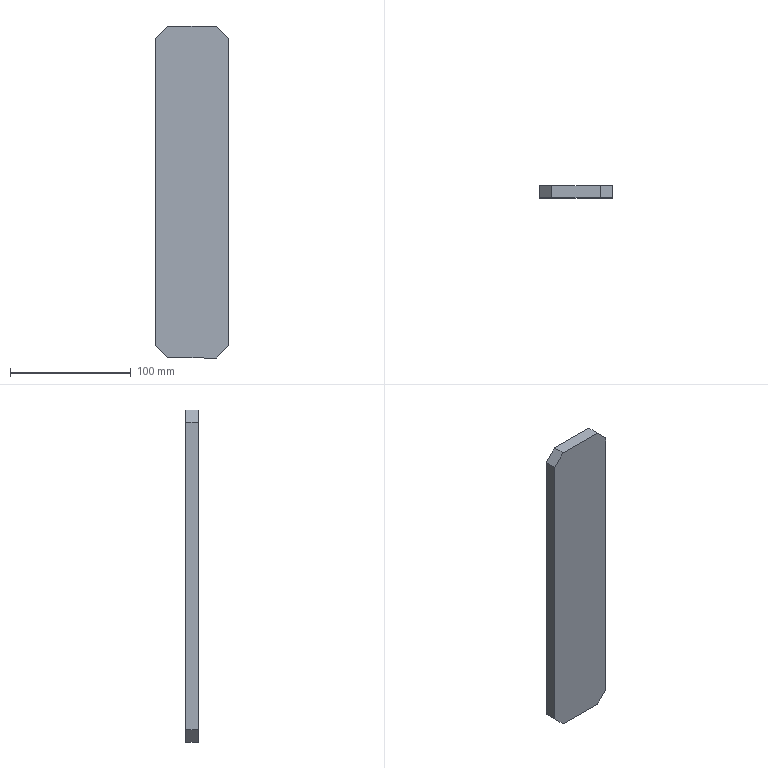Part | SolidWorks | features BaseBody 1 | 1 solid | 10 faces | box 60 x 10 x 275 mm | volume 163000 mm3 | plane 10
STEP:
#1=CARTESIAN_POINT('',(650.,52.,448.));
#2=VERTEX_POINT('',#1);
#3=CARTESIAN_POINT('',(640.,52.,438.));
#4=VERTEX_POINT('',#3);
#5=CARTESIAN_POINT('',(650.,52.,448.));
#6=DIRECTION('',(-0.7071,0.,-0.7071));
#7=VECTOR('',#6,1000.);
#8=LINE('',#5,#7);
#9=EDGE_CURVE('',#2,#4,#8,.T.);
#10=ORIENTED_EDGE('',*,*,#9,.T.);
#11=CARTESIAN_POINT('',(640.,52.,183.));
#12=VERTEX_POINT('',#11);
#13=CARTESIAN_POINT('',(640.,52.,-1110.));
#14=DIRECTION('',(0.,0.,-1.));
#15=VECTOR('',#14,1000.);
#16=LINE('',#13,#15);
#17=EDGE_CURVE('',#4,#12,#16,.T.);
#18=ORIENTED_EDGE('',*,*,#17,.T.);
#19=CARTESIAN_POINT('',(650.,52.,173.));
#20=VERTEX_POINT('',#19);
#21=CARTESIAN_POINT('',(640.,52.,183.));
#22=DIRECTION('',(0.7071,0.,-0.7071));
#23=VECTOR('',#22,1000.);
#24=LINE('',#21,#23);
#25=EDGE_CURVE('',#12,#20,#24,.T.);
#26=ORIENTED_EDGE('',*,*,#25,.T.);
#27=CARTESIAN_POINT('',(690.,52.,173.));
#28=VERTEX_POINT('',#27);
#29=CARTESIAN_POINT('',(1039.958,52.,173.));
#30=DIRECTION('',(1.,0.,0.));
#31=VECTOR('',#30,1000.);
#32=LINE('',#29,#31);
#33=EDGE_CURVE('',#20,#28,#32,.T.);
#34=ORIENTED_EDGE('',*,*,#33,.T.);
#35=CARTESIAN_POINT('',(700.,52.,183.));
#36=VERTEX_POINT('',#35);
#37=CARTESIAN_POINT('',(690.,52.,173.));
#38=DIRECTION('',(0.7071,0.,0.7071));
#39=VECTOR('',#38,1000.);
#40=LINE('',#37,#39);
#41=EDGE_CURVE('',#28,#36,#40,.T.);
#42=ORIENTED_EDGE('',*,*,#41,.T.);
#43=CARTESIAN_POINT('',(700.,52.,438.));
#44=VERTEX_POINT('',#43);
#45=CARTESIAN_POINT('',(700.,52.,-1110.));
#46=DIRECTION('',(0.,0.,1.));
#47=VECTOR('',#46,1000.);
#48=LINE('',#45,#47);
#49=EDGE_CURVE('',#36,#44,#48,.T.);
#50=ORIENTED_EDGE('',*,*,#49,.T.);
#51=CARTESIAN_POINT('',(690.,52.,448.));
#52=VERTEX_POINT('',#51);
#53=CARTESIAN_POINT('',(700.,52.,438.));
#54=DIRECTION('',(-0.7071,0.,0.7071));
#55=VECTOR('',#54,1000.);
#56=LINE('',#53,#55);
#57=EDGE_CURVE('',#44,#52,#56,.T.);
#58=ORIENTED_EDGE('',*,*,#57,.T.);
#59=CARTESIAN_POINT('',(1039.958,52.,448.));
#60=DIRECTION('',(-1.,0.,0.));
#61=VECTOR('',#60,1000.);
#62=LINE('',#59,#61);
#63=EDGE_CURVE('',#52,#2,#62,.T.);
#64=ORIENTED_EDGE('',*,*,#63,.T.);
#65=EDGE_LOOP('',(#10,#18,#26,#34,#42,#50,#58,#64));
#66=FACE_OUTER_BOUND('',#65,.T.);
#67=CARTESIAN_POINT('',(1039.958,52.,-1110.));
#68=DIRECTION('',(0.,-1.,0.));
#69=DIRECTION('',(0.,0.,-1.));
#70=AXIS2_PLACEMENT_3D('',#67,#68,#69);
#71=PLANE('',#70);
#72=ADVANCED_FACE('',(#66),#71,.T.);
#73=ORIENTED_EDGE('',*,*,#17,.F.);
#74=CARTESIAN_POINT('',(640.,62.,438.));
#75=VERTEX_POINT('',#74);
#76=CARTESIAN_POINT('',(640.,44.,438.));
#77=DIRECTION('',(0.,-1.,0.));
#78=VECTOR('',#77,1000.);
#79=LINE('',#76,#78);
#80=EDGE_CURVE('',#75,#4,#79,.T.);
#81=ORIENTED_EDGE('',*,*,#80,.F.);
#82=CARTESIAN_POINT('',(640.,62.,183.));
#83=VERTEX_POINT('',#82);
#84=CARTESIAN_POINT('',(640.,62.,530.));
#85=DIRECTION('',(0.,0.,1.));
#86=VECTOR('',#85,1000.);
#87=LINE('',#84,#86);
#88=EDGE_CURVE('',#83,#75,#87,.T.);
#89=ORIENTED_EDGE('',*,*,#88,.F.);
#90=CARTESIAN_POINT('',(640.,44.,183.));
#91=DIRECTION('',(0.,1.,0.));
#92=VECTOR('',#91,1000.);
#93=LINE('',#90,#92);
#94=EDGE_CURVE('',#12,#83,#93,.T.);
#95=ORIENTED_EDGE('',*,*,#94,.F.);
#96=EDGE_LOOP('',(#73,#81,#89,#95));
#97=FACE_OUTER_BOUND('',#96,.T.);
#98=CARTESIAN_POINT('',(640.,44.,530.));
#99=DIRECTION('',(1.,0.,0.));
#100=DIRECTION('',(0.,0.,-1.));
#101=AXIS2_PLACEMENT_3D('',#98,#99,#100);
#102=PLANE('',#101);
#103=ADVANCED_FACE('',(#97),#102,.F.);
#104=CARTESIAN_POINT('',(650.,62.,448.));
#105=VERTEX_POINT('',#104);
#106=CARTESIAN_POINT('',(640.,62.,438.));
#107=DIRECTION('',(0.7071,0.,0.7071));
#108=VECTOR('',#107,1000.);
#109=LINE('',#106,#108);
#110=EDGE_CURVE('',#75,#105,#109,.T.);
#111=ORIENTED_EDGE('',*,*,#110,.F.);
#112=ORIENTED_EDGE('',*,*,#80,.T.);
#113=ORIENTED_EDGE('',*,*,#9,.F.);
#114=CARTESIAN_POINT('',(650.,44.,448.));
#115=DIRECTION('',(0.,-1.,0.));
#116=VECTOR('',#115,1000.);
#117=LINE('',#114,#116);
#118=EDGE_CURVE('',#105,#2,#117,.T.);
#119=ORIENTED_EDGE('',*,*,#118,.F.);
#120=EDGE_LOOP('',(#111,#112,#113,#119));
#121=FACE_OUTER_BOUND('',#120,.T.);
#122=CARTESIAN_POINT('',(640.,44.,438.));
#123=DIRECTION('',(0.7071,0.,-0.7071));
#124=DIRECTION('',(-0.7071,0.,-0.7071));
#125=AXIS2_PLACEMENT_3D('',#122,#123,#124);
#126=PLANE('',#125);
#127=ADVANCED_FACE('',(#121),#126,.F.);
#128=ORIENTED_EDGE('',*,*,#63,.F.);
#129=CARTESIAN_POINT('',(690.,62.,448.));
#130=VERTEX_POINT('',#129);
#131=CARTESIAN_POINT('',(690.,52.,448.));
#132=DIRECTION('',(0.,-1.,0.));
#133=VECTOR('',#132,1000.);
#134=LINE('',#131,#133);
#135=EDGE_CURVE('',#130,#52,#134,.T.);
#136=ORIENTED_EDGE('',*,*,#135,.F.);
#137=CARTESIAN_POINT('',(644.958,62.,448.));
#138=DIRECTION('',(1.,0.,0.));
#139=VECTOR('',#138,1000.);
#140=LINE('',#137,#139);
#141=EDGE_CURVE('',#105,#130,#140,.T.);
#142=ORIENTED_EDGE('',*,*,#141,.F.);
#143=ORIENTED_EDGE('',*,*,#118,.T.);
#144=EDGE_LOOP('',(#128,#136,#142,#143));
#145=FACE_OUTER_BOUND('',#144,.T.);
#146=CARTESIAN_POINT('',(644.958,52.,448.));
#147=DIRECTION('',(0.,0.,-1.));
#148=DIRECTION('',(-1.,0.,0.));
#149=AXIS2_PLACEMENT_3D('',#146,#147,#148);
#150=PLANE('',#149);
#151=ADVANCED_FACE('',(#145),#150,.F.);
#152=CARTESIAN_POINT('',(700.,62.,438.));
#153=VERTEX_POINT('',#152);
#154=CARTESIAN_POINT('',(690.,62.,448.));
#155=DIRECTION('',(0.7071,0.,-0.7071));
#156=VECTOR('',#155,1000.);
#157=LINE('',#154,#156);
#158=EDGE_CURVE('',#130,#153,#157,.T.);
#159=ORIENTED_EDGE('',*,*,#158,.F.);
#160=ORIENTED_EDGE('',*,*,#135,.T.);
#161=ORIENTED_EDGE('',*,*,#57,.F.);
#162=CARTESIAN_POINT('',(700.,52.,438.));
#163=DIRECTION('',(0.,-1.,0.));
#164=VECTOR('',#163,1000.);
#165=LINE('',#162,#164);
#166=EDGE_CURVE('',#153,#44,#165,.T.);
#167=ORIENTED_EDGE('',*,*,#166,.F.);
#168=EDGE_LOOP('',(#159,#160,#161,#167));
#169=FACE_OUTER_BOUND('',#168,.T.);
#170=CARTESIAN_POINT('',(690.,52.,448.));
#171=DIRECTION('',(-0.7071,0.,-0.7071));
#172=DIRECTION('',(-0.7071,0.,0.7071));
#173=AXIS2_PLACEMENT_3D('',#170,#171,#172);
#174=PLANE('',#173);
#175=ADVANCED_FACE('',(#169),#174,.F.);
#176=CARTESIAN_POINT('',(700.,62.,183.));
#177=VERTEX_POINT('',#176);
#178=CARTESIAN_POINT('',(700.,62.,530.));
#179=DIRECTION('',(0.,0.,-1.));
#180=VECTOR('',#179,1000.);
#181=LINE('',#178,#180);
#182=EDGE_CURVE('',#153,#177,#181,.T.);
#183=ORIENTED_EDGE('',*,*,#182,.F.);
#184=ORIENTED_EDGE('',*,*,#166,.T.);
#185=ORIENTED_EDGE('',*,*,#49,.F.);
#186=CARTESIAN_POINT('',(700.,0.,183.));
#187=DIRECTION('',(0.,-1.,0.));
#188=VECTOR('',#187,1000.);
#189=LINE('',#186,#188);
#190=EDGE_CURVE('',#177,#36,#189,.T.);
#191=ORIENTED_EDGE('',*,*,#190,.F.);
#192=EDGE_LOOP('',(#183,#184,#185,#191));
#193=FACE_OUTER_BOUND('',#192,.T.);
#194=CARTESIAN_POINT('',(700.,0.,530.));
#195=DIRECTION('',(-1.,0.,0.));
#196=DIRECTION('',(0.,0.,1.));
#197=AXIS2_PLACEMENT_3D('',#194,#195,#196);
#198=PLANE('',#197);
#199=ADVANCED_FACE('',(#193),#198,.F.);
#200=ORIENTED_EDGE('',*,*,#190,.T.);
#201=ORIENTED_EDGE('',*,*,#41,.F.);
#202=CARTESIAN_POINT('',(690.,62.,173.));
#203=VERTEX_POINT('',#202);
#204=CARTESIAN_POINT('',(690.,0.,173.));
#205=DIRECTION('',(0.,1.,0.));
#206=VECTOR('',#205,1000.);
#207=LINE('',#204,#206);
#208=EDGE_CURVE('',#28,#203,#207,.T.);
#209=ORIENTED_EDGE('',*,*,#208,.T.);
#210=CARTESIAN_POINT('',(700.,62.,183.));
#211=DIRECTION('',(0.7071,0.,0.7071));
#212=VECTOR('',#211,1000.);
#213=LINE('',#210,#212);
#214=EDGE_CURVE('',#203,#177,#213,.T.);
#215=ORIENTED_EDGE('',*,*,#214,.T.);
#216=EDGE_LOOP('',(#200,#201,#209,#215));
#217=FACE_OUTER_BOUND('',#216,.T.);
#218=CARTESIAN_POINT('',(700.,0.,183.));
#219=DIRECTION('',(0.7071,0.,-0.7071));
#220=DIRECTION('',(-0.7071,0.,-0.7071));
#221=AXIS2_PLACEMENT_3D('',#218,#219,#220);
#222=PLANE('',#221);
#223=ADVANCED_FACE('',(#217),#222,.T.);
#224=ORIENTED_EDGE('',*,*,#208,.F.);
#225=ORIENTED_EDGE('',*,*,#33,.F.);
#226=CARTESIAN_POINT('',(650.,62.,173.));
#227=VERTEX_POINT('',#226);
#228=CARTESIAN_POINT('',(650.,83.661,173.));
#229=DIRECTION('',(0.,1.,0.));
#230=VECTOR('',#229,1000.);
#231=LINE('',#228,#230);
#232=EDGE_CURVE('',#20,#227,#231,.T.);
#233=ORIENTED_EDGE('',*,*,#232,.T.);
#234=CARTESIAN_POINT('',(655.558,62.,173.));
#235=DIRECTION('',(1.,0.,0.));
#236=VECTOR('',#235,1000.);
#237=LINE('',#234,#236);
#238=EDGE_CURVE('',#227,#203,#237,.T.);
#239=ORIENTED_EDGE('',*,*,#238,.T.);
#240=EDGE_LOOP('',(#224,#225,#233,#239));
#241=FACE_OUTER_BOUND('',#240,.T.);
#242=CARTESIAN_POINT('',(655.558,83.661,173.));
#243=DIRECTION('',(0.,0.,-1.));
#244=DIRECTION('',(-1.,0.,0.));
#245=AXIS2_PLACEMENT_3D('',#242,#243,#244);
#246=PLANE('',#245);
#247=ADVANCED_FACE('',(#241),#246,.T.);
#248=ORIENTED_EDGE('',*,*,#232,.F.);
#249=ORIENTED_EDGE('',*,*,#25,.F.);
#250=ORIENTED_EDGE('',*,*,#94,.T.);
#251=CARTESIAN_POINT('',(650.,62.,173.));
#252=DIRECTION('',(0.7071,0.,-0.7071));
#253=VECTOR('',#252,1000.);
#254=LINE('',#251,#253);
#255=EDGE_CURVE('',#83,#227,#254,.T.);
#256=ORIENTED_EDGE('',*,*,#255,.T.);
#257=EDGE_LOOP('',(#248,#249,#250,#256));
#258=FACE_OUTER_BOUND('',#257,.T.);
#259=CARTESIAN_POINT('',(650.,83.661,173.));
#260=DIRECTION('',(-0.7071,0.,-0.7071));
#261=DIRECTION('',(-0.7071,0.,0.7071));
#262=AXIS2_PLACEMENT_3D('',#259,#260,#261);
#263=PLANE('',#262);
#264=ADVANCED_FACE('',(#258),#263,.T.);
#265=ORIENTED_EDGE('',*,*,#88,.T.);
#266=ORIENTED_EDGE('',*,*,#110,.T.);
#267=ORIENTED_EDGE('',*,*,#141,.T.);
#268=ORIENTED_EDGE('',*,*,#158,.T.);
#269=ORIENTED_EDGE('',*,*,#182,.T.);
#270=ORIENTED_EDGE('',*,*,#214,.F.);
#271=ORIENTED_EDGE('',*,*,#238,.F.);
#272=ORIENTED_EDGE('',*,*,#255,.F.);
#273=EDGE_LOOP('',(#265,#266,#267,#268,#269,#270,#271,#272));
#274=FACE_OUTER_BOUND('',#273,.T.);
#275=CARTESIAN_POINT('',(1039.958,62.,-1110.));
#276=DIRECTION('',(0.,-1.,0.));
#277=DIRECTION('',(0.,0.,-1.));
#278=AXIS2_PLACEMENT_3D('',#275,#276,#277);
#279=PLANE('',#278);
#280=ADVANCED_FACE('',(#274),#279,.F.);
#281=CLOSED_SHELL('',(#72,#103,#127,#151,#175,#199,#223,#247,#264,#280));
#282=MANIFOLD_SOLID_BREP('',#281);
#283=CARTESIAN_POINT('',(0.,0.,0.));
#284=DIRECTION('',(0.,0.,1.));
#285=DIRECTION('',(1.,0.,0.));
#286=AXIS2_PLACEMENT_3D('',#283,#284,#285);
#287=(LENGTH_UNIT()NAMED_UNIT(*)SI_UNIT(.MILLI.,.METRE.));
#288=UNCERTAINTY_MEASURE_WITH_UNIT(LENGTH_MEASURE(0.00001),#287,'','');
#289=(NAMED_UNIT(*)PLANE_ANGLE_UNIT()SI_UNIT($,.RADIAN.));
#290=(NAMED_UNIT(*)SI_UNIT($,.STERADIAN.)SOLID_ANGLE_UNIT());
#291=(GEOMETRIC_REPRESENTATION_CONTEXT(3)GLOBAL_UNCERTAINTY_ASSIGNED_CONTEXT((#288))GLOBAL_UNIT_ASSIGNED_CONTEXT((#287,#289,#290))REPRESENTATION_CONTEXT('',''));
#292=ADVANCED_BREP_SHAPE_REPRESENTATION('',(#282,#286),#291);